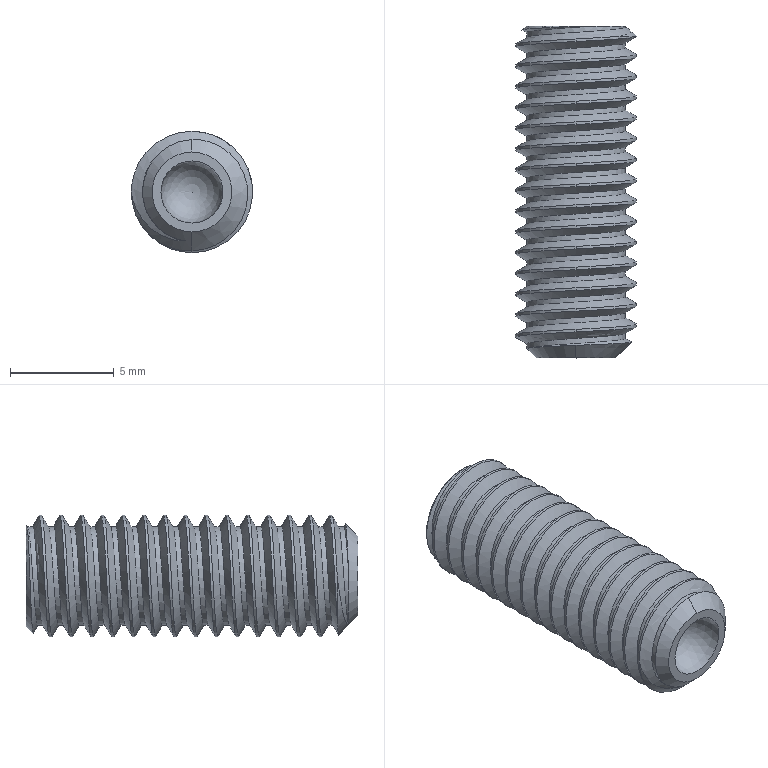Part | STEP file | Plug M6_16 | 1 solid | 50 faces | box 5.85 x 16 x 5.85 mm | volume 295.252 mm3 | cylinder 30 | plane 9 | cone 5 | sphere 3 | spline 3 | commonest cylinder face diameters 5.85 x30